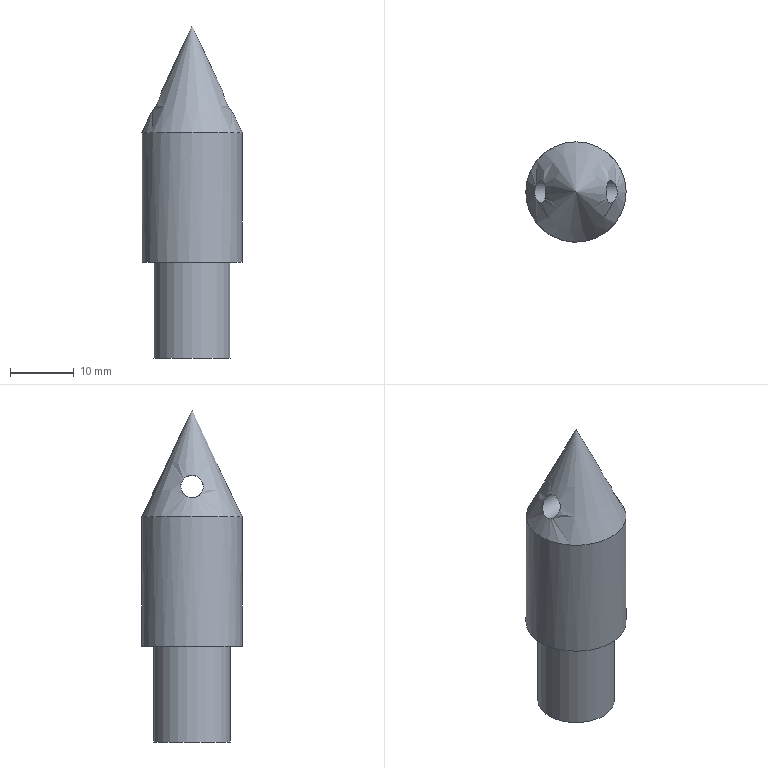Part | NX | features solid 2 | 1 solid | 6 faces | box 15.7 x 15.7 x 52 mm | volume 6599 mm3 | cylinder 3 | plane 2 | cone 1 | commonest cylinder face diameters 3.5 x1 12 x1 15.7 x1
STEP:
#1=CARTESIAN_POINT('',(354.998,16.349,-25.));
#2=VERTEX_POINT('',#1);
#3=CARTESIAN_POINT('',(354.998,10.349,-25.));
#4=DIRECTION('',(0.,0.,-1.));
#5=DIRECTION('',(0.,1.,0.));
#6=AXIS2_PLACEMENT_3D('',#3,#4,#5);
#7=CIRCLE('',#6,6.);
#8=EDGE_CURVE('',#2,#2,#7,.T.);
#9=ORIENTED_EDGE('',*,*,#8,.T.);
#10=EDGE_LOOP('',(#9));
#11=FACE_BOUND('',#10,.T.);
#12=CARTESIAN_POINT('',(348.998,10.349,-25.));
#13=DIRECTION('',(0.,0.,1.));
#14=DIRECTION('',(0.,-1.,0.));
#15=AXIS2_PLACEMENT_3D('',#12,#13,#14);
#16=PLANE('',#15);
#17=ADVANCED_FACE('',(#11),#16,.F.);
#18=ORIENTED_EDGE('',*,*,#8,.F.);
#19=EDGE_LOOP('',(#18));
#20=FACE_BOUND('',#19,.T.);
#21=CARTESIAN_POINT('',(354.998,16.349,-10.));
#22=VERTEX_POINT('',#21);
#23=CARTESIAN_POINT('',(354.998,10.349,-10.));
#24=DIRECTION('',(0.,0.,-1.));
#25=DIRECTION('',(0.,1.,0.));
#26=AXIS2_PLACEMENT_3D('',#23,#24,#25);
#27=CIRCLE('',#26,6.);
#28=EDGE_CURVE('',#22,#22,#27,.T.);
#29=ORIENTED_EDGE('',*,*,#28,.T.);
#30=EDGE_LOOP('',(#29));
#31=FACE_BOUND('',#30,.T.);
#32=CARTESIAN_POINT('',(354.998,10.349,-25.));
#33=DIRECTION('',(0.,0.,-1.));
#34=DIRECTION('',(0.,1.,0.));
#35=AXIS2_PLACEMENT_3D('',#32,#33,#34);
#36=CYLINDRICAL_SURFACE('',#35,6.);
#37=ADVANCED_FACE('',(#20,#31),#36,.T.);
#38=ORIENTED_EDGE('',*,*,#28,.F.);
#39=EDGE_LOOP('',(#38));
#40=FACE_BOUND('',#39,.T.);
#41=CARTESIAN_POINT('',(362.848,10.349,-10.));
#42=VERTEX_POINT('',#41);
#43=CARTESIAN_POINT('',(354.998,10.349,-10.));
#44=DIRECTION('',(0.,0.,1.));
#45=DIRECTION('',(1.,0.,0.));
#46=AXIS2_PLACEMENT_3D('',#43,#44,#45);
#47=CIRCLE('',#46,7.85);
#48=EDGE_CURVE('',#42,#42,#47,.F.);
#49=ORIENTED_EDGE('',*,*,#48,.T.);
#50=EDGE_LOOP('',(#49));
#51=FACE_BOUND('',#50,.T.);
#52=CARTESIAN_POINT('',(346.998,10.349,-10.));
#53=DIRECTION('',(0.,0.,1.));
#54=DIRECTION('',(0.,-1.,0.));
#55=AXIS2_PLACEMENT_3D('',#52,#53,#54);
#56=PLANE('',#55);
#57=ADVANCED_FACE('',(#40,#51),#56,.F.);
#58=ORIENTED_EDGE('',*,*,#48,.F.);
#59=EDGE_LOOP('',(#58));
#60=FACE_BOUND('',#59,.T.);
#61=CARTESIAN_POINT('',(347.148,10.349,10.319));
#62=VERTEX_POINT('',#61);
#63=CARTESIAN_POINT('',(354.998,10.349,10.319));
#64=DIRECTION('',(0.,0.,-1.));
#65=DIRECTION('',(-1.,0.,0.));
#66=AXIS2_PLACEMENT_3D('',#63,#64,#65);
#67=CIRCLE('',#66,7.85);
#68=EDGE_CURVE('',#62,#62,#67,.T.);
#69=ORIENTED_EDGE('',*,*,#68,.T.);
#70=EDGE_LOOP('',(#69));
#71=FACE_BOUND('',#70,.T.);
#72=CARTESIAN_POINT('',(354.998,10.349,-25.));
#73=DIRECTION('',(0.,0.,-1.));
#74=DIRECTION('',(0.,1.,0.));
#75=AXIS2_PLACEMENT_3D('',#72,#73,#74);
#76=CYLINDRICAL_SURFACE('',#75,7.85);
#77=ADVANCED_FACE('',(#60,#71),#76,.T.);
#78=CARTESIAN_POINT('',(348.71,11.253,13.501));
#79=VERTEX_POINT('',#78);
#80=CARTESIAN_POINT('',(348.433,9.781,13.122));
#81=CARTESIAN_POINT('',(348.612,11.392,13.357));
#82=CARTESIAN_POINT('',(349.381,12.17,14.459));
#83=CARTESIAN_POINT('',(350.046,12.099,15.848));
#84=CARTESIAN_POINT('',(350.19,10.9,16.893));
#85=CARTESIAN_POINT('',(350.192,9.31,16.67));
#86=CARTESIAN_POINT('',(349.871,8.457,15.372));
#87=CARTESIAN_POINT('',(349.118,8.695,14.058));
#88=CARTESIAN_POINT('',(348.433,9.781,13.122));
#89=CARTESIAN_POINT('',(348.612,11.392,13.357));
#90=CARTESIAN_POINT('',(349.381,12.17,14.459));
#91=B_SPLINE_CURVE_WITH_KNOTS('',3,(#80,#81,#82,#83,#84,#85,#86,#87,#88,#89,#90),.UNSPECIFIED.,.T.,.F.,(1,1,1,1,1,1,1,1,1,1,1,1,1,1,1),(-0.00434,-0.002893,-0.001447,0.,0.001447,0.002893,0.00434,0.005787,0.007234,0.00868,0.01013,0.01157,0.01302,0.01447,0.01591),.UNSPECIFIED.);
#92=EDGE_CURVE('',#79,#79,#91,.T.);
#93=ORIENTED_EDGE('',*,*,#92,.T.);
#94=EDGE_LOOP('',(#93));
#95=FACE_BOUND('',#94,.T.);
#96=CARTESIAN_POINT('',(361.143,11.526,13.705));
#97=VERTEX_POINT('',#96);
#98=CARTESIAN_POINT('',(360.42,12.245,14.784));
#99=CARTESIAN_POINT('',(361.203,11.673,13.601));
#100=CARTESIAN_POINT('',(361.628,10.216,13.038));
#101=CARTESIAN_POINT('',(361.081,8.878,13.769));
#102=CARTESIAN_POINT('',(360.301,8.436,15.004));
#103=CARTESIAN_POINT('',(359.828,8.974,16.397));
#104=CARTESIAN_POINT('',(359.811,10.478,16.968));
#105=CARTESIAN_POINT('',(359.859,11.889,16.207));
#106=CARTESIAN_POINT('',(360.42,12.245,14.784));
#107=CARTESIAN_POINT('',(361.203,11.673,13.601));
#108=CARTESIAN_POINT('',(361.628,10.216,13.038));
#109=B_SPLINE_CURVE_WITH_KNOTS('',3,(#98,#99,#100,#101,#102,#103,#104,#105,#106,#107,#108),.UNSPECIFIED.,.T.,.F.,(1,1,1,1,1,1,1,1,1,1,1,1,1,1,1),(-0.004351,-0.0029,-0.00145,0.,0.00145,0.0029,0.004351,0.005801,0.007251,0.008701,0.01015,0.0116,0.01305,0.0145,0.01595),.UNSPECIFIED.);
#110=EDGE_CURVE('',#97,#97,#109,.T.);
#111=ORIENTED_EDGE('',*,*,#110,.T.);
#112=EDGE_LOOP('',(#111));
#113=FACE_BOUND('',#112,.T.);
#114=ORIENTED_EDGE('',*,*,#68,.F.);
#115=EDGE_LOOP('',(#114));
#116=FACE_BOUND('',#115,.T.);
#117=CARTESIAN_POINT('',(354.998,10.349,27.));
#118=VERTEX_POINT('',#117);
#119=VERTEX_LOOP('',#118);
#120=FACE_BOUND('',#119,.T.);
#121=CARTESIAN_POINT('',(354.998,10.349,27.));
#122=DIRECTION('',(0.,0.,-1.));
#123=DIRECTION('',(0.,1.,0.));
#124=AXIS2_PLACEMENT_3D('',#121,#122,#123);
#125=CONICAL_SURFACE('',#124,0.,0.4398);
#126=ADVANCED_FACE('',(#95,#113,#116,#120),#125,.T.);
#127=ORIENTED_EDGE('',*,*,#110,.F.);
#128=EDGE_LOOP('',(#127));
#129=FACE_BOUND('',#128,.T.);
#130=ORIENTED_EDGE('',*,*,#92,.F.);
#131=EDGE_LOOP('',(#130));
#132=FACE_BOUND('',#131,.T.);
#133=CARTESIAN_POINT('',(-88.002,10.349,15.));
#134=DIRECTION('',(1.,0.,0.));
#135=DIRECTION('',(0.,1.,0.));
#136=AXIS2_PLACEMENT_3D('',#133,#134,#135);
#137=CYLINDRICAL_SURFACE('',#136,1.75);
#138=ADVANCED_FACE('',(#129,#132),#137,.F.);
#139=CLOSED_SHELL('',(#17,#37,#57,#77,#126,#138));
#140=MANIFOLD_SOLID_BREP('',#139);
#141=(LENGTH_UNIT()NAMED_UNIT(*)SI_UNIT(.MILLI.,.METRE.));
#142=UNCERTAINTY_MEASURE_WITH_UNIT(LENGTH_MEASURE(0.0508),#141,'','');
#143=(NAMED_UNIT(*)PLANE_ANGLE_UNIT()SI_UNIT($,.RADIAN.));
#144=(NAMED_UNIT(*)SI_UNIT($,.STERADIAN.)SOLID_ANGLE_UNIT());
#145=(GEOMETRIC_REPRESENTATION_CONTEXT(3)GLOBAL_UNCERTAINTY_ASSIGNED_CONTEXT((#142))GLOBAL_UNIT_ASSIGNED_CONTEXT((#141,#143,#144))REPRESENTATION_CONTEXT('',''));
#146=ADVANCED_BREP_SHAPE_REPRESENTATION('',(#140),#145);